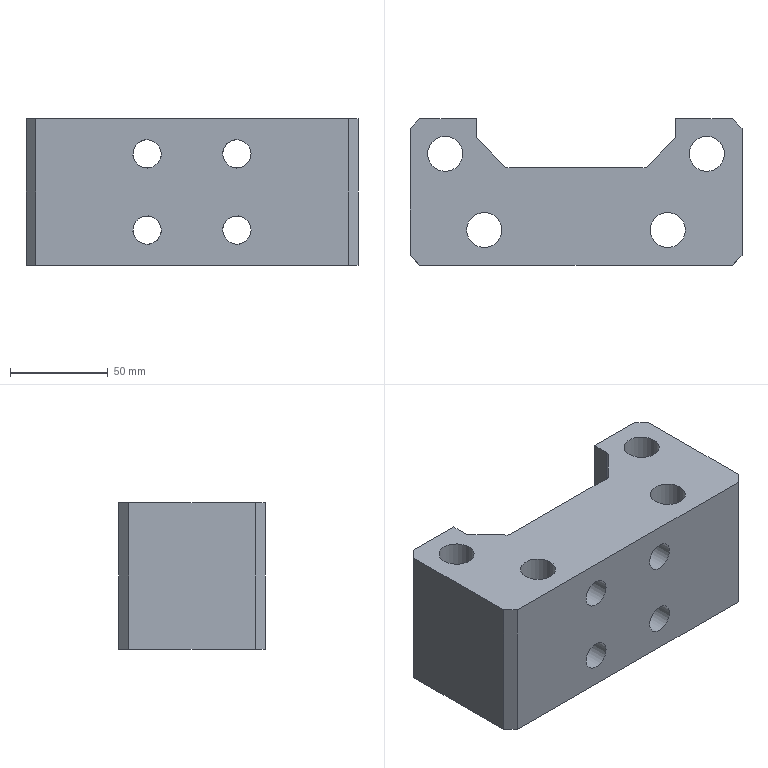Part | NX | features UB-6 2 | 1 solid | 48 faces | box 170 x 75 x 75 mm | volume 622690 mm3 | plane 22 | cylinder 20 | cone 6 | commonest cylinder face diameters 6 x4 14.5 x4 18 x4 26 x4 10.506 x2 12 x2
STEP:
#1=CARTESIAN_POINT('',(3330.594,-689.122,948.466));
#2=VERTEX_POINT('',#1);
#3=CARTESIAN_POINT('',(3330.594,-689.122,955.716));
#4=DIRECTION('',(0.,-1.,0.));
#5=DIRECTION('',(0.,0.,-1.));
#6=AXIS2_PLACEMENT_3D('',#3,#4,#5);
#7=CIRCLE('',#6,7.25);
#8=EDGE_CURVE('',#2,#2,#7,.T.);
#9=ORIENTED_EDGE('',*,*,#8,.F.);
#10=EDGE_LOOP('',(#9));
#11=FACE_BOUND('',#10,.T.);
#12=CARTESIAN_POINT('',(3284.594,-689.122,948.466));
#13=VERTEX_POINT('',#12);
#14=CARTESIAN_POINT('',(3284.594,-689.122,955.716));
#15=DIRECTION('',(0.,-1.,0.));
#16=DIRECTION('',(0.,0.,-1.));
#17=AXIS2_PLACEMENT_3D('',#14,#15,#16);
#18=CIRCLE('',#17,7.25);
#19=EDGE_CURVE('',#13,#13,#18,.T.);
#20=ORIENTED_EDGE('',*,*,#19,.F.);
#21=EDGE_LOOP('',(#20));
#22=FACE_BOUND('',#21,.T.);
#23=CARTESIAN_POINT('',(3227.594,-689.122,973.716));
#24=VERTEX_POINT('',#23);
#25=CARTESIAN_POINT('',(3387.594,-689.122,973.716));
#26=VERTEX_POINT('',#25);
#27=CARTESIAN_POINT('',(3237.747,-689.122,973.716));
#28=DIRECTION('',(1.,0.,0.));
#29=VECTOR('',#28,1000.);
#30=LINE('',#27,#29);
#31=EDGE_CURVE('',#24,#26,#30,.T.);
#32=ORIENTED_EDGE('',*,*,#31,.F.);
#33=CARTESIAN_POINT('',(3227.594,-689.122,898.716));
#34=VERTEX_POINT('',#33);
#35=CARTESIAN_POINT('',(3227.594,-689.122,973.716));
#36=DIRECTION('',(0.,0.,1.));
#37=VECTOR('',#36,1000.);
#38=LINE('',#35,#37);
#39=EDGE_CURVE('',#34,#24,#38,.T.);
#40=ORIENTED_EDGE('',*,*,#39,.F.);
#41=CARTESIAN_POINT('',(3387.594,-689.122,898.716));
#42=VERTEX_POINT('',#41);
#43=CARTESIAN_POINT('',(3645.094,-689.122,898.716));
#44=DIRECTION('',(1.,0.,0.));
#45=VECTOR('',#44,1000.);
#46=LINE('',#43,#45);
#47=EDGE_CURVE('',#34,#42,#46,.T.);
#48=ORIENTED_EDGE('',*,*,#47,.T.);
#49=CARTESIAN_POINT('',(3387.594,-689.122,1023.116));
#50=DIRECTION('',(0.,0.,-1.));
#51=VECTOR('',#50,1000.);
#52=LINE('',#49,#51);
#53=EDGE_CURVE('',#26,#42,#52,.T.);
#54=ORIENTED_EDGE('',*,*,#53,.F.);
#55=EDGE_LOOP('',(#32,#40,#48,#54));
#56=FACE_BOUND('',#55,.T.);
#57=CARTESIAN_POINT('',(3284.594,-689.122,909.466));
#58=VERTEX_POINT('',#57);
#59=CARTESIAN_POINT('',(3284.594,-689.122,916.716));
#60=DIRECTION('',(0.,-1.,0.));
#61=DIRECTION('',(0.,0.,-1.));
#62=AXIS2_PLACEMENT_3D('',#59,#60,#61);
#63=CIRCLE('',#62,7.25);
#64=EDGE_CURVE('',#58,#58,#63,.T.);
#65=ORIENTED_EDGE('',*,*,#64,.F.);
#66=EDGE_LOOP('',(#65));
#67=FACE_BOUND('',#66,.T.);
#68=CARTESIAN_POINT('',(3330.594,-689.122,909.466));
#69=VERTEX_POINT('',#68);
#70=CARTESIAN_POINT('',(3330.594,-689.122,916.716));
#71=DIRECTION('',(0.,-1.,0.));
#72=DIRECTION('',(0.,0.,-1.));
#73=AXIS2_PLACEMENT_3D('',#70,#71,#72);
#74=CIRCLE('',#73,7.25);
#75=EDGE_CURVE('',#69,#69,#74,.T.);
#76=ORIENTED_EDGE('',*,*,#75,.F.);
#77=EDGE_LOOP('',(#76));
#78=FACE_BOUND('',#77,.T.);
#79=CARTESIAN_POINT('',(4847.709,-689.122,1023.116));
#80=DIRECTION('',(0.,1.,0.));
#81=DIRECTION('',(0.,0.,-1.));
#82=AXIS2_PLACEMENT_3D('',#79,#80,#81);
#83=PLANE('',#82);
#84=ADVANCED_FACE('',(#11,#22,#56,#67,#78),#83,.F.);
#85=CARTESIAN_POINT('',(3269.594,-671.122,973.716));
#86=VERTEX_POINT('',#85);
#87=CARTESIAN_POINT('',(3260.594,-671.122,973.716));
#88=DIRECTION('',(0.,0.,-1.));
#89=DIRECTION('',(1.,0.,0.));
#90=AXIS2_PLACEMENT_3D('',#87,#88,#89);
#91=CIRCLE('',#90,9.);
#92=EDGE_CURVE('',#86,#86,#91,.T.);
#93=ORIENTED_EDGE('',*,*,#92,.T.);
#94=EDGE_LOOP('',(#93));
#95=FACE_BOUND('',#94,.T.);
#96=CARTESIAN_POINT('',(3383.594,-632.122,973.716));
#97=VERTEX_POINT('',#96);
#98=CARTESIAN_POINT('',(3374.594,-632.122,973.716));
#99=DIRECTION('',(0.,0.,-1.));
#100=DIRECTION('',(1.,0.,0.));
#101=AXIS2_PLACEMENT_3D('',#98,#99,#100);
#102=CIRCLE('',#101,9.);
#103=EDGE_CURVE('',#97,#97,#102,.T.);
#104=ORIENTED_EDGE('',*,*,#103,.T.);
#105=EDGE_LOOP('',(#104));
#106=FACE_BOUND('',#105,.T.);
#107=CARTESIAN_POINT('',(3249.594,-632.122,973.716));
#108=VERTEX_POINT('',#107);
#109=CARTESIAN_POINT('',(3240.594,-632.122,973.716));
#110=DIRECTION('',(0.,0.,-1.));
#111=DIRECTION('',(1.,0.,0.));
#112=AXIS2_PLACEMENT_3D('',#109,#110,#111);
#113=CIRCLE('',#112,9.);
#114=EDGE_CURVE('',#108,#108,#113,.T.);
#115=ORIENTED_EDGE('',*,*,#114,.T.);
#116=EDGE_LOOP('',(#115));
#117=FACE_BOUND('',#116,.T.);
#118=CARTESIAN_POINT('',(3363.594,-671.122,973.716));
#119=VERTEX_POINT('',#118);
#120=CARTESIAN_POINT('',(3354.594,-671.122,973.716));
#121=DIRECTION('',(0.,0.,-1.));
#122=DIRECTION('',(1.,0.,0.));
#123=AXIS2_PLACEMENT_3D('',#120,#121,#122);
#124=CIRCLE('',#123,9.);
#125=EDGE_CURVE('',#119,#119,#124,.T.);
#126=ORIENTED_EDGE('',*,*,#125,.T.);
#127=EDGE_LOOP('',(#126));
#128=FACE_BOUND('',#127,.T.);
#129=CARTESIAN_POINT('',(3345.075,-637.498,973.716));
#130=VERTEX_POINT('',#129);
#131=CARTESIAN_POINT('',(3341.156,-639.122,973.716));
#132=VERTEX_POINT('',#131);
#133=CARTESIAN_POINT('',(3342.304,-636.35,973.716));
#134=DIRECTION('',(0.,0.,-1.));
#135=DIRECTION('',(1.,0.,0.));
#136=AXIS2_PLACEMENT_3D('',#133,#134,#135);
#137=CIRCLE('',#136,3.);
#138=EDGE_CURVE('',#130,#132,#137,.T.);
#139=ORIENTED_EDGE('',*,*,#138,.T.);
#140=CARTESIAN_POINT('',(3274.032,-639.122,973.716));
#141=VERTEX_POINT('',#140);
#142=CARTESIAN_POINT('',(3307.594,-639.122,973.716));
#143=DIRECTION('',(1.,0.,0.));
#144=VECTOR('',#143,1000.);
#145=LINE('',#142,#144);
#146=EDGE_CURVE('',#141,#132,#145,.T.);
#147=ORIENTED_EDGE('',*,*,#146,.F.);
#148=CARTESIAN_POINT('',(3270.112,-637.498,973.716));
#149=VERTEX_POINT('',#148);
#150=CARTESIAN_POINT('',(3272.884,-636.35,973.716));
#151=DIRECTION('',(0.,0.,1.));
#152=DIRECTION('',(1.,0.,0.));
#153=AXIS2_PLACEMENT_3D('',#150,#151,#152);
#154=CIRCLE('',#153,3.);
#155=EDGE_CURVE('',#149,#141,#154,.T.);
#156=ORIENTED_EDGE('',*,*,#155,.F.);
#157=CARTESIAN_POINT('',(3257.473,-624.859,973.716));
#158=VERTEX_POINT('',#157);
#159=CARTESIAN_POINT('',(3435.992,-803.378,973.716));
#160=DIRECTION('',(-0.7071,0.7071,0.));
#161=VECTOR('',#160,1000.);
#162=LINE('',#159,#161);
#163=EDGE_CURVE('',#149,#158,#162,.T.);
#164=ORIENTED_EDGE('',*,*,#163,.T.);
#165=CARTESIAN_POINT('',(3256.594,-622.737,973.716));
#166=VERTEX_POINT('',#165);
#167=CARTESIAN_POINT('',(3259.594,-622.737,973.716));
#168=DIRECTION('',(0.,0.,1.));
#169=DIRECTION('',(1.,0.,0.));
#170=AXIS2_PLACEMENT_3D('',#167,#168,#169);
#171=CIRCLE('',#170,3.);
#172=EDGE_CURVE('',#166,#158,#171,.T.);
#173=ORIENTED_EDGE('',*,*,#172,.F.);
#174=CARTESIAN_POINT('',(3256.594,-614.122,973.716));
#175=VERTEX_POINT('',#174);
#176=CARTESIAN_POINT('',(3256.594,-1016.622,973.716));
#177=DIRECTION('',(0.,1.,0.));
#178=VECTOR('',#177,1000.);
#179=LINE('',#176,#178);
#180=EDGE_CURVE('',#166,#175,#179,.T.);
#181=ORIENTED_EDGE('',*,*,#180,.T.);
#182=CARTESIAN_POINT('',(3227.594,-614.122,973.716));
#183=VERTEX_POINT('',#182);
#184=CARTESIAN_POINT('',(4385.094,-614.122,973.716));
#185=DIRECTION('',(-1.,0.,0.));
#186=VECTOR('',#185,1000.);
#187=LINE('',#184,#186);
#188=EDGE_CURVE('',#175,#183,#187,.T.);
#189=ORIENTED_EDGE('',*,*,#188,.T.);
#190=CARTESIAN_POINT('',(3222.594,-619.122,973.716));
#191=VERTEX_POINT('',#190);
#192=CARTESIAN_POINT('',(3023.92,-817.796,973.716));
#193=DIRECTION('',(0.7071,0.7071,0.));
#194=VECTOR('',#193,1000.);
#195=LINE('',#192,#194);
#196=EDGE_CURVE('',#191,#183,#195,.T.);
#197=ORIENTED_EDGE('',*,*,#196,.F.);
#198=CARTESIAN_POINT('',(3222.594,-684.122,973.716));
#199=VERTEX_POINT('',#198);
#200=CARTESIAN_POINT('',(3222.594,-1016.622,973.716));
#201=DIRECTION('',(0.,1.,0.));
#202=VECTOR('',#201,1000.);
#203=LINE('',#200,#202);
#204=EDGE_CURVE('',#199,#191,#203,.T.);
#205=ORIENTED_EDGE('',*,*,#204,.F.);
#206=CARTESIAN_POINT('',(3388.92,-850.449,973.716));
#207=DIRECTION('',(-0.7071,0.7071,0.));
#208=VECTOR('',#207,1000.);
#209=LINE('',#206,#208);
#210=EDGE_CURVE('',#24,#199,#209,.T.);
#211=ORIENTED_EDGE('',*,*,#210,.F.);
#212=ORIENTED_EDGE('',*,*,#31,.T.);
#213=CARTESIAN_POINT('',(3392.594,-684.122,973.716));
#214=VERTEX_POINT('',#213);
#215=CARTESIAN_POINT('',(3156.42,-920.296,973.716));
#216=DIRECTION('',(-0.7071,-0.7071,0.));
#217=VECTOR('',#216,1000.);
#218=LINE('',#215,#217);
#219=EDGE_CURVE('',#214,#26,#218,.T.);
#220=ORIENTED_EDGE('',*,*,#219,.F.);
#221=CARTESIAN_POINT('',(3392.594,-619.122,973.716));
#222=VERTEX_POINT('',#221);
#223=CARTESIAN_POINT('',(3392.594,-699.122,973.716));
#224=DIRECTION('',(0.,-1.,0.));
#225=VECTOR('',#224,1000.);
#226=LINE('',#223,#225);
#227=EDGE_CURVE('',#222,#214,#226,.T.);
#228=ORIENTED_EDGE('',*,*,#227,.F.);
#229=CARTESIAN_POINT('',(3387.594,-614.122,973.716));
#230=VERTEX_POINT('',#229);
#231=CARTESIAN_POINT('',(3521.42,-747.949,973.716));
#232=DIRECTION('',(0.7071,-0.7071,0.));
#233=VECTOR('',#232,1000.);
#234=LINE('',#231,#233);
#235=EDGE_CURVE('',#230,#222,#234,.T.);
#236=ORIENTED_EDGE('',*,*,#235,.F.);
#237=CARTESIAN_POINT('',(3358.594,-614.122,973.716));
#238=VERTEX_POINT('',#237);
#239=CARTESIAN_POINT('',(4387.594,-614.122,973.716));
#240=DIRECTION('',(-1.,0.,0.));
#241=VECTOR('',#240,1000.);
#242=LINE('',#239,#241);
#243=EDGE_CURVE('',#230,#238,#242,.T.);
#244=ORIENTED_EDGE('',*,*,#243,.T.);
#245=CARTESIAN_POINT('',(3358.594,-622.737,973.716));
#246=VERTEX_POINT('',#245);
#247=CARTESIAN_POINT('',(3358.594,-656.622,973.716));
#248=DIRECTION('',(0.,1.,0.));
#249=VECTOR('',#248,1000.);
#250=LINE('',#247,#249);
#251=EDGE_CURVE('',#246,#238,#250,.T.);
#252=ORIENTED_EDGE('',*,*,#251,.F.);
#253=CARTESIAN_POINT('',(3357.715,-624.859,973.716));
#254=VERTEX_POINT('',#253);
#255=CARTESIAN_POINT('',(3355.594,-622.737,973.716));
#256=DIRECTION('',(0.,0.,1.));
#257=DIRECTION('',(1.,0.,0.));
#258=AXIS2_PLACEMENT_3D('',#255,#256,#257);
#259=CIRCLE('',#258,3.);
#260=EDGE_CURVE('',#254,#246,#259,.T.);
#261=ORIENTED_EDGE('',*,*,#260,.F.);
#262=CARTESIAN_POINT('',(3340.523,-642.051,973.716));
#263=DIRECTION('',(-0.7071,-0.7071,0.));
#264=VECTOR('',#263,1000.);
#265=LINE('',#262,#264);
#266=EDGE_CURVE('',#254,#130,#265,.T.);
#267=ORIENTED_EDGE('',*,*,#266,.T.);
#268=EDGE_LOOP('',(#139,#147,#156,#164,#173,#181,#189,#197,#205,#211,#212,#220,#228,#236,#244,#252,#261,#267));
#269=FACE_BOUND('',#268,.T.);
#270=CARTESIAN_POINT('',(3237.747,-1016.622,973.716));
#271=DIRECTION('',(0.,0.,1.));
#272=DIRECTION('',(-1.,0.,0.));
#273=AXIS2_PLACEMENT_3D('',#270,#271,#272);
#274=PLANE('',#273);
#275=ADVANCED_FACE('',(#95,#106,#117,#128,#269),#274,.T.);
#276=CARTESIAN_POINT('',(3231.594,-656.622,898.716));
#277=VERTEX_POINT('',#276);
#278=CARTESIAN_POINT('',(3237.594,-656.622,898.716));
#279=DIRECTION('',(0.,0.,-1.));
#280=DIRECTION('',(-1.,0.,0.));
#281=AXIS2_PLACEMENT_3D('',#278,#279,#280);
#282=CIRCLE('',#281,6.);
#283=EDGE_CURVE('',#277,#277,#282,.T.);
#284=ORIENTED_EDGE('',*,*,#283,.F.);
#285=EDGE_LOOP('',(#284));
#286=FACE_BOUND('',#285,.T.);
#287=CARTESIAN_POINT('',(3383.594,-656.622,898.716));
#288=VERTEX_POINT('',#287);
#289=CARTESIAN_POINT('',(3377.594,-656.622,898.716));
#290=DIRECTION('',(0.,0.,1.));
#291=DIRECTION('',(1.,0.,0.));
#292=AXIS2_PLACEMENT_3D('',#289,#290,#291);
#293=CIRCLE('',#292,6.);
#294=EDGE_CURVE('',#288,#288,#293,.T.);
#295=ORIENTED_EDGE('',*,*,#294,.T.);
#296=EDGE_LOOP('',(#295));
#297=FACE_BOUND('',#296,.T.);
#298=CARTESIAN_POINT('',(3273.594,-671.122,898.716));
#299=VERTEX_POINT('',#298);
#300=CARTESIAN_POINT('',(3260.594,-671.122,898.716));
#301=DIRECTION('',(0.,0.,-1.));
#302=DIRECTION('',(1.,0.,0.));
#303=AXIS2_PLACEMENT_3D('',#300,#301,#302);
#304=CIRCLE('',#303,13.);
#305=EDGE_CURVE('',#299,#299,#304,.T.);
#306=ORIENTED_EDGE('',*,*,#305,.F.);
#307=EDGE_LOOP('',(#306));
#308=FACE_BOUND('',#307,.T.);
#309=CARTESIAN_POINT('',(3387.594,-632.122,898.716));
#310=VERTEX_POINT('',#309);
#311=CARTESIAN_POINT('',(3374.594,-632.122,898.716));
#312=DIRECTION('',(0.,0.,-1.));
#313=DIRECTION('',(1.,0.,0.));
#314=AXIS2_PLACEMENT_3D('',#311,#312,#313);
#315=CIRCLE('',#314,13.);
#316=EDGE_CURVE('',#310,#310,#315,.T.);
#317=ORIENTED_EDGE('',*,*,#316,.F.);
#318=EDGE_LOOP('',(#317));
#319=FACE_BOUND('',#318,.T.);
#320=CARTESIAN_POINT('',(3253.594,-632.122,898.716));
#321=VERTEX_POINT('',#320);
#322=CARTESIAN_POINT('',(3240.594,-632.122,898.716));
#323=DIRECTION('',(0.,0.,-1.));
#324=DIRECTION('',(1.,0.,0.));
#325=AXIS2_PLACEMENT_3D('',#322,#323,#324);
#326=CIRCLE('',#325,13.);
#327=EDGE_CURVE('',#321,#321,#326,.T.);
#328=ORIENTED_EDGE('',*,*,#327,.F.);
#329=EDGE_LOOP('',(#328));
#330=FACE_BOUND('',#329,.T.);
#331=CARTESIAN_POINT('',(3367.594,-671.122,898.716));
#332=VERTEX_POINT('',#331);
#333=CARTESIAN_POINT('',(3354.594,-671.122,898.716));
#334=DIRECTION('',(0.,0.,-1.));
#335=DIRECTION('',(1.,0.,0.));
#336=AXIS2_PLACEMENT_3D('',#333,#334,#335);
#337=CIRCLE('',#336,13.);
#338=EDGE_CURVE('',#332,#332,#337,.T.);
#339=ORIENTED_EDGE('',*,*,#338,.F.);
#340=EDGE_LOOP('',(#339));
#341=FACE_BOUND('',#340,.T.);
#342=CARTESIAN_POINT('',(3357.715,-624.859,898.716));
#343=VERTEX_POINT('',#342);
#344=CARTESIAN_POINT('',(3345.075,-637.498,898.716));
#345=VERTEX_POINT('',#344);
#346=CARTESIAN_POINT('',(3340.523,-642.051,898.716));
#347=DIRECTION('',(-0.7071,-0.7071,0.));
#348=VECTOR('',#347,1000.);
#349=LINE('',#346,#348);
#350=EDGE_CURVE('',#343,#345,#349,.T.);
#351=ORIENTED_EDGE('',*,*,#350,.F.);
#352=CARTESIAN_POINT('',(3358.594,-622.737,898.716));
#353=VERTEX_POINT('',#352);
#354=CARTESIAN_POINT('',(3355.594,-622.737,898.716));
#355=DIRECTION('',(0.,0.,-1.));
#356=DIRECTION('',(1.,0.,0.));
#357=AXIS2_PLACEMENT_3D('',#354,#355,#356);
#358=CIRCLE('',#357,3.);
#359=EDGE_CURVE('',#353,#343,#358,.T.);
#360=ORIENTED_EDGE('',*,*,#359,.F.);
#361=CARTESIAN_POINT('',(3358.594,-614.122,898.716));
#362=VERTEX_POINT('',#361);
#363=CARTESIAN_POINT('',(3358.594,-1419.122,898.716));
#364=DIRECTION('',(0.,-1.,0.));
#365=VECTOR('',#364,1000.);
#366=LINE('',#363,#365);
#367=EDGE_CURVE('',#362,#353,#366,.T.);
#368=ORIENTED_EDGE('',*,*,#367,.F.);
#369=CARTESIAN_POINT('',(3387.594,-614.122,898.716));
#370=VERTEX_POINT('',#369);
#371=CARTESIAN_POINT('',(3660.094,-614.122,898.716));
#372=DIRECTION('',(1.,0.,0.));
#373=VECTOR('',#372,1000.);
#374=LINE('',#371,#373);
#375=EDGE_CURVE('',#362,#370,#374,.T.);
#376=ORIENTED_EDGE('',*,*,#375,.T.);
#377=CARTESIAN_POINT('',(3392.594,-619.122,898.716));
#378=VERTEX_POINT('',#377);
#379=CARTESIAN_POINT('',(3392.594,-619.122,898.716));
#380=DIRECTION('',(-0.7071,0.7071,0.));
#381=VECTOR('',#380,1000.);
#382=LINE('',#379,#381);
#383=EDGE_CURVE('',#378,#370,#382,.T.);
#384=ORIENTED_EDGE('',*,*,#383,.F.);
#385=CARTESIAN_POINT('',(3392.594,-684.122,898.716));
#386=VERTEX_POINT('',#385);
#387=CARTESIAN_POINT('',(3392.594,-1419.122,898.716));
#388=DIRECTION('',(0.,1.,0.));
#389=VECTOR('',#388,1000.);
#390=LINE('',#387,#389);
#391=EDGE_CURVE('',#386,#378,#390,.T.);
#392=ORIENTED_EDGE('',*,*,#391,.F.);
#393=CARTESIAN_POINT('',(3387.594,-689.122,898.716));
#394=DIRECTION('',(0.7071,0.7071,0.));
#395=VECTOR('',#394,1000.);
#396=LINE('',#393,#395);
#397=EDGE_CURVE('',#42,#386,#396,.T.);
#398=ORIENTED_EDGE('',*,*,#397,.F.);
#399=ORIENTED_EDGE('',*,*,#47,.F.);
#400=CARTESIAN_POINT('',(3222.594,-684.122,898.716));
#401=VERTEX_POINT('',#400);
#402=CARTESIAN_POINT('',(3222.594,-684.122,898.716));
#403=DIRECTION('',(0.7071,-0.7071,0.));
#404=VECTOR('',#403,1000.);
#405=LINE('',#402,#404);
#406=EDGE_CURVE('',#401,#34,#405,.T.);
#407=ORIENTED_EDGE('',*,*,#406,.F.);
#408=CARTESIAN_POINT('',(3222.594,-619.122,898.716));
#409=VERTEX_POINT('',#408);
#410=CARTESIAN_POINT('',(3222.594,-1419.122,898.716));
#411=DIRECTION('',(0.,1.,0.));
#412=VECTOR('',#411,1000.);
#413=LINE('',#410,#412);
#414=EDGE_CURVE('',#401,#409,#413,.T.);
#415=ORIENTED_EDGE('',*,*,#414,.T.);
#416=CARTESIAN_POINT('',(3227.594,-614.122,898.716));
#417=VERTEX_POINT('',#416);
#418=CARTESIAN_POINT('',(3227.594,-614.122,898.716));
#419=DIRECTION('',(-0.7071,-0.7071,0.));
#420=VECTOR('',#419,1000.);
#421=LINE('',#418,#420);
#422=EDGE_CURVE('',#417,#409,#421,.T.);
#423=ORIENTED_EDGE('',*,*,#422,.F.);
#424=CARTESIAN_POINT('',(3256.594,-614.122,898.716));
#425=VERTEX_POINT('',#424);
#426=CARTESIAN_POINT('',(4385.094,-614.122,898.716));
#427=DIRECTION('',(-1.,0.,0.));
#428=VECTOR('',#427,1000.);
#429=LINE('',#426,#428);
#430=EDGE_CURVE('',#425,#417,#429,.T.);
#431=ORIENTED_EDGE('',*,*,#430,.F.);
#432=CARTESIAN_POINT('',(3256.594,-622.737,898.716));
#433=VERTEX_POINT('',#432);
#434=CARTESIAN_POINT('',(3256.594,-656.622,898.716));
#435=DIRECTION('',(0.,-1.,0.));
#436=VECTOR('',#435,1000.);
#437=LINE('',#434,#436);
#438=EDGE_CURVE('',#425,#433,#437,.T.);
#439=ORIENTED_EDGE('',*,*,#438,.T.);
#440=CARTESIAN_POINT('',(3257.473,-624.859,898.716));
#441=VERTEX_POINT('',#440);
#442=CARTESIAN_POINT('',(3259.594,-622.737,898.716));
#443=DIRECTION('',(0.,0.,-1.));
#444=DIRECTION('',(1.,0.,0.));
#445=AXIS2_PLACEMENT_3D('',#442,#443,#444);
#446=CIRCLE('',#445,3.);
#447=EDGE_CURVE('',#441,#433,#446,.T.);
#448=ORIENTED_EDGE('',*,*,#447,.F.);
#449=CARTESIAN_POINT('',(3270.112,-637.498,898.716));
#450=VERTEX_POINT('',#449);
#451=CARTESIAN_POINT('',(3840.915,-1208.301,898.716));
#452=DIRECTION('',(-0.7071,0.7071,0.));
#453=VECTOR('',#452,1000.);
#454=LINE('',#451,#453);
#455=EDGE_CURVE('',#450,#441,#454,.T.);
#456=ORIENTED_EDGE('',*,*,#455,.F.);
#457=CARTESIAN_POINT('',(3274.032,-639.122,898.716));
#458=VERTEX_POINT('',#457);
#459=CARTESIAN_POINT('',(3272.884,-636.35,898.716));
#460=DIRECTION('',(0.,0.,-1.));
#461=DIRECTION('',(1.,0.,0.));
#462=AXIS2_PLACEMENT_3D('',#459,#460,#461);
#463=CIRCLE('',#462,3.);
#464=EDGE_CURVE('',#458,#450,#463,.T.);
#465=ORIENTED_EDGE('',*,*,#464,.F.);
#466=CARTESIAN_POINT('',(3341.156,-639.122,898.716));
#467=VERTEX_POINT('',#466);
#468=CARTESIAN_POINT('',(3645.094,-639.122,898.716));
#469=DIRECTION('',(-1.,0.,0.));
#470=VECTOR('',#469,1000.);
#471=LINE('',#468,#470);
#472=EDGE_CURVE('',#467,#458,#471,.T.);
#473=ORIENTED_EDGE('',*,*,#472,.F.);
#474=CARTESIAN_POINT('',(3342.304,-636.35,898.716));
#475=DIRECTION('',(0.,0.,-1.));
#476=DIRECTION('',(1.,0.,0.));
#477=AXIS2_PLACEMENT_3D('',#474,#475,#476);
#478=CIRCLE('',#477,3.);
#479=EDGE_CURVE('',#345,#467,#478,.T.);
#480=ORIENTED_EDGE('',*,*,#479,.F.);
#481=EDGE_LOOP('',(#351,#360,#368,#376,#384,#392,#398,#399,#407,#415,#423,#431,#439,#448,#456,#465,#473,#480));
#482=FACE_BOUND('',#481,.T.);
#483=CARTESIAN_POINT('',(3645.094,-1419.122,898.716));
#484=DIRECTION('',(0.,0.,1.));
#485=DIRECTION('',(-1.,0.,0.));
#486=AXIS2_PLACEMENT_3D('',#483,#484,#485);
#487=PLANE('',#486);
#488=ADVANCED_FACE('',(#286,#297,#308,#319,#330,#341,#482),#487,.F.);
#489=ORIENTED_EDGE('',*,*,#455,.T.);
#490=CARTESIAN_POINT('',(3257.473,-624.859,898.716));
#491=DIRECTION('',(0.,0.,-1.));
#492=VECTOR('',#491,1000.);
#493=LINE('',#490,#492);
#494=EDGE_CURVE('',#158,#441,#493,.T.);
#495=ORIENTED_EDGE('',*,*,#494,.F.);
#496=ORIENTED_EDGE('',*,*,#163,.F.);
#497=CARTESIAN_POINT('',(3270.112,-637.498,973.716));
#498=DIRECTION('',(0.,0.,1.));
#499=VECTOR('',#498,1000.);
#500=LINE('',#497,#499);
#501=EDGE_CURVE('',#450,#149,#500,.T.);
#502=ORIENTED_EDGE('',*,*,#501,.F.);
#503=EDGE_LOOP('',(#489,#495,#496,#502));
#504=FACE_BOUND('',#503,.T.);
#505=CARTESIAN_POINT('',(3289.665,-657.051,583.116));
#506=DIRECTION('',(-0.7071,-0.7071,0.));
#507=DIRECTION('',(0.,0.,1.));
#508=AXIS2_PLACEMENT_3D('',#505,#506,#507);
#509=PLANE('',#508);
#510=ADVANCED_FACE('',(#504),#509,.F.);
#511=CARTESIAN_POINT('',(3345.075,-637.498,898.716));
#512=DIRECTION('',(0.,0.,1.));
#513=VECTOR('',#512,1000.);
#514=LINE('',#511,#513);
#515=EDGE_CURVE('',#345,#130,#514,.T.);
#516=ORIENTED_EDGE('',*,*,#515,.T.);
#517=ORIENTED_EDGE('',*,*,#266,.F.);
#518=CARTESIAN_POINT('',(3357.715,-624.859,943.716));
#519=DIRECTION('',(0.,0.,1.));
#520=VECTOR('',#519,1000.);
#521=LINE('',#518,#520);
#522=EDGE_CURVE('',#343,#254,#521,.T.);
#523=ORIENTED_EDGE('',*,*,#522,.F.);
#524=ORIENTED_EDGE('',*,*,#350,.T.);
#525=EDGE_LOOP('',(#516,#517,#523,#524));
#526=FACE_BOUND('',#525,.T.);
#527=CARTESIAN_POINT('',(3340.523,-642.051,943.716));
#528=DIRECTION('',(-0.7071,0.7071,0.));
#529=DIRECTION('',(-0.7071,-0.7071,0.));
#530=AXIS2_PLACEMENT_3D('',#527,#528,#529);
#531=PLANE('',#530);
#532=ADVANCED_FACE('',(#526),#531,.T.);
#533=ORIENTED_EDGE('',*,*,#375,.F.);
#534=CARTESIAN_POINT('',(3358.594,-614.122,938.716));
#535=DIRECTION('',(0.,0.,-1.));
#536=VECTOR('',#535,1000.);
#537=LINE('',#534,#536);
#538=EDGE_CURVE('',#238,#362,#537,.T.);
#539=ORIENTED_EDGE('',*,*,#538,.F.);
#540=ORIENTED_EDGE('',*,*,#243,.F.);
#541=CARTESIAN_POINT('',(3387.594,-614.122,973.716));
#542=DIRECTION('',(0.,0.,1.));
#543=VECTOR('',#542,1000.);
#544=LINE('',#541,#543);
#545=EDGE_CURVE('',#370,#230,#544,.T.);
#546=ORIENTED_EDGE('',*,*,#545,.F.);
#547=EDGE_LOOP('',(#533,#539,#540,#546));
#548=FACE_BOUND('',#547,.T.);
#549=CARTESIAN_POINT('',(4387.594,-614.122,858.716));
#550=DIRECTION('',(0.,1.,0.));
#551=DIRECTION('',(-1.,0.,0.));
#552=AXIS2_PLACEMENT_3D('',#549,#550,#551);
#553=PLANE('',#552);
#554=ADVANCED_FACE('',(#548),#553,.T.);
#555=ORIENTED_EDGE('',*,*,#227,.T.);
#556=CARTESIAN_POINT('',(3392.594,-684.122,1068.116));
#557=DIRECTION('',(0.,0.,1.));
#558=VECTOR('',#557,1000.);
#559=LINE('',#556,#558);
#560=EDGE_CURVE('',#386,#214,#559,.T.);
#561=ORIENTED_EDGE('',*,*,#560,.F.);
#562=ORIENTED_EDGE('',*,*,#391,.T.);
#563=CARTESIAN_POINT('',(3392.594,-619.122,898.716));
#564=DIRECTION('',(0.,0.,-1.));
#565=VECTOR('',#564,1000.);
#566=LINE('',#563,#565);
#567=EDGE_CURVE('',#222,#378,#566,.T.);
#568=ORIENTED_EDGE('',*,*,#567,.F.);
#569=EDGE_LOOP('',(#555,#561,#562,#568));
#570=FACE_BOUND('',#569,.T.);
#571=CARTESIAN_POINT('',(3392.594,-699.122,1068.116));
#572=DIRECTION('',(-1.,0.,0.));
#573=DIRECTION('',(0.,0.,-1.));
#574=AXIS2_PLACEMENT_3D('',#571,#572,#573);
#575=PLANE('',#574);
#576=ADVANCED_FACE('',(#570),#575,.F.);
#577=ORIENTED_EDGE('',*,*,#251,.T.);
#578=ORIENTED_EDGE('',*,*,#538,.T.);
#579=ORIENTED_EDGE('',*,*,#367,.T.);
#580=CARTESIAN_POINT('',(3358.594,-622.737,938.716));
#581=DIRECTION('',(0.,0.,-1.));
#582=VECTOR('',#581,1000.);
#583=LINE('',#580,#582);
#584=EDGE_CURVE('',#246,#353,#583,.T.);
#585=ORIENTED_EDGE('',*,*,#584,.F.);
#586=EDGE_LOOP('',(#577,#578,#579,#585));
#587=FACE_BOUND('',#586,.T.);
#588=CARTESIAN_POINT('',(3358.594,-656.622,938.716));
#589=DIRECTION('',(1.,0.,0.));
#590=DIRECTION('',(0.,0.,1.));
#591=AXIS2_PLACEMENT_3D('',#588,#589,#590);
#592=PLANE('',#591);
#593=ADVANCED_FACE('',(#587),#592,.F.);
#594=ORIENTED_EDGE('',*,*,#204,.T.);
#595=CARTESIAN_POINT('',(3222.594,-619.122,1068.116));
#596=DIRECTION('',(0.,0.,1.));
#597=VECTOR('',#596,1000.);
#598=LINE('',#595,#597);
#599=EDGE_CURVE('',#409,#191,#598,.T.);
#600=ORIENTED_EDGE('',*,*,#599,.F.);
#601=ORIENTED_EDGE('',*,*,#414,.F.);
#602=CARTESIAN_POINT('',(3222.594,-684.122,898.716));
#603=DIRECTION('',(0.,0.,-1.));
#604=VECTOR('',#603,1000.);
#605=LINE('',#602,#604);
#606=EDGE_CURVE('',#199,#401,#605,.T.);
#607=ORIENTED_EDGE('',*,*,#606,.F.);
#608=EDGE_LOOP('',(#594,#600,#601,#607));
#609=FACE_BOUND('',#608,.T.);
#610=CARTESIAN_POINT('',(3222.594,-699.122,1068.116));
#611=DIRECTION('',(-1.,0.,0.));
#612=DIRECTION('',(0.,0.,-1.));
#613=AXIS2_PLACEMENT_3D('',#610,#611,#612);
#614=PLANE('',#613);
#615=ADVANCED_FACE('',(#609),#614,.T.);
#616=ORIENTED_EDGE('',*,*,#188,.F.);
#617=CARTESIAN_POINT('',(3256.594,-614.122,858.716));
#618=DIRECTION('',(0.,0.,-1.));
#619=VECTOR('',#618,1000.);
#620=LINE('',#617,#619);
#621=EDGE_CURVE('',#175,#425,#620,.T.);
#622=ORIENTED_EDGE('',*,*,#621,.T.);
#623=ORIENTED_EDGE('',*,*,#430,.T.);
#624=CARTESIAN_POINT('',(3227.594,-614.122,858.716));
#625=DIRECTION('',(0.,0.,-1.));
#626=VECTOR('',#625,1000.);
#627=LINE('',#624,#626);
#628=EDGE_CURVE('',#183,#417,#627,.T.);
#629=ORIENTED_EDGE('',*,*,#628,.F.);
#630=EDGE_LOOP('',(#616,#622,#623,#629));
#631=FACE_BOUND('',#630,.T.);
#632=CARTESIAN_POINT('',(4385.094,-614.122,858.716));
#633=DIRECTION('',(0.,1.,0.));
#634=DIRECTION('',(-1.,0.,0.));
#635=AXIS2_PLACEMENT_3D('',#632,#633,#634);
#636=PLANE('',#635);
#637=ADVANCED_FACE('',(#631),#636,.T.);
#638=ORIENTED_EDGE('',*,*,#438,.F.);
#639=ORIENTED_EDGE('',*,*,#621,.F.);
#640=ORIENTED_EDGE('',*,*,#180,.F.);
#641=CARTESIAN_POINT('',(3256.594,-622.737,998.716));
#642=DIRECTION('',(0.,0.,1.));
#643=VECTOR('',#642,1000.);
#644=LINE('',#641,#643);
#645=EDGE_CURVE('',#433,#166,#644,.T.);
#646=ORIENTED_EDGE('',*,*,#645,.F.);
#647=EDGE_LOOP('',(#638,#639,#640,#646));
#648=FACE_BOUND('',#647,.T.);
#649=CARTESIAN_POINT('',(3256.594,-656.622,938.716));
#650=DIRECTION('',(-1.,0.,0.));
#651=DIRECTION('',(0.,0.,-1.));
#652=AXIS2_PLACEMENT_3D('',#649,#650,#651);
#653=PLANE('',#652);
#654=ADVANCED_FACE('',(#648),#653,.F.);
#655=ORIENTED_EDGE('',*,*,#172,.T.);
#656=ORIENTED_EDGE('',*,*,#494,.T.);
#657=ORIENTED_EDGE('',*,*,#447,.T.);
#658=ORIENTED_EDGE('',*,*,#645,.T.);
#659=EDGE_LOOP('',(#655,#656,#657,#658));
#660=FACE_BOUND('',#659,.T.);
#661=CARTESIAN_POINT('',(3259.594,-622.737,583.116));
#662=DIRECTION('',(0.,0.,1.));
#663=DIRECTION('',(-1.,0.,0.));
#664=AXIS2_PLACEMENT_3D('',#661,#662,#663);
#665=CYLINDRICAL_SURFACE('',#664,3.);
#666=ADVANCED_FACE('',(#660),#665,.F.);
#667=ORIENTED_EDGE('',*,*,#359,.T.);
#668=ORIENTED_EDGE('',*,*,#522,.T.);
#669=ORIENTED_EDGE('',*,*,#260,.T.);
#670=ORIENTED_EDGE('',*,*,#584,.T.);
#671=EDGE_LOOP('',(#667,#668,#669,#670));
#672=FACE_BOUND('',#671,.T.);
#673=CARTESIAN_POINT('',(3355.594,-622.737,943.716));
#674=DIRECTION('',(0.,0.,1.));
#675=DIRECTION('',(-1.,0.,0.));
#676=AXIS2_PLACEMENT_3D('',#673,#674,#675);
#677=CYLINDRICAL_SURFACE('',#676,3.);
#678=ADVANCED_FACE('',(#672),#677,.F.);
#679=CARTESIAN_POINT('',(3292.594,-639.122,955.716));
#680=VERTEX_POINT('',#679);
#681=CARTESIAN_POINT('',(3284.594,-639.122,955.716));
#682=DIRECTION('',(0.,-1.,0.));
#683=DIRECTION('',(1.,0.,0.));
#684=AXIS2_PLACEMENT_3D('',#681,#682,#683);
#685=CIRCLE('',#684,8.);
#686=EDGE_CURVE('',#680,#680,#685,.T.);
#687=ORIENTED_EDGE('',*,*,#686,.T.);
#688=EDGE_LOOP('',(#687));
#689=FACE_BOUND('',#688,.T.);
#690=CARTESIAN_POINT('',(3338.594,-639.122,916.716));
#691=VERTEX_POINT('',#690);
#692=CARTESIAN_POINT('',(3330.594,-639.122,916.716));
#693=DIRECTION('',(0.,-1.,0.));
#694=DIRECTION('',(1.,0.,0.));
#695=AXIS2_PLACEMENT_3D('',#692,#693,#694);
#696=CIRCLE('',#695,8.);
#697=EDGE_CURVE('',#691,#691,#696,.T.);
#698=ORIENTED_EDGE('',*,*,#697,.T.);
#699=EDGE_LOOP('',(#698));
#700=FACE_BOUND('',#699,.T.);
#701=CARTESIAN_POINT('',(3292.594,-639.122,916.716));
#702=VERTEX_POINT('',#701);
#703=CARTESIAN_POINT('',(3284.594,-639.122,916.716));
#704=DIRECTION('',(0.,-1.,0.));
#705=DIRECTION('',(1.,0.,0.));
#706=AXIS2_PLACEMENT_3D('',#703,#704,#705);
#707=CIRCLE('',#706,8.);
#708=EDGE_CURVE('',#702,#702,#707,.T.);
#709=ORIENTED_EDGE('',*,*,#708,.T.);
#710=EDGE_LOOP('',(#709));
#711=FACE_BOUND('',#710,.T.);
#712=CARTESIAN_POINT('',(3338.594,-639.122,955.716));
#713=VERTEX_POINT('',#712);
#714=CARTESIAN_POINT('',(3330.594,-639.122,955.716));
#715=DIRECTION('',(0.,-1.,0.));
#716=DIRECTION('',(1.,0.,0.));
#717=AXIS2_PLACEMENT_3D('',#714,#715,#716);
#718=CIRCLE('',#717,8.);
#719=EDGE_CURVE('',#713,#713,#718,.T.);
#720=ORIENTED_EDGE('',*,*,#719,.T.);
#721=EDGE_LOOP('',(#720));
#722=FACE_BOUND('',#721,.T.);
#723=ORIENTED_EDGE('',*,*,#472,.T.);
#724=CARTESIAN_POINT('',(3274.032,-639.122,973.716));
#725=DIRECTION('',(0.,0.,-1.));
#726=VECTOR('',#725,1000.);
#727=LINE('',#724,#726);
#728=EDGE_CURVE('',#141,#458,#727,.T.);
#729=ORIENTED_EDGE('',*,*,#728,.F.);
#730=ORIENTED_EDGE('',*,*,#146,.T.);
#731=CARTESIAN_POINT('',(3341.156,-639.122,898.716));
#732=DIRECTION('',(0.,0.,1.));
#733=VECTOR('',#732,1000.);
#734=LINE('',#731,#733);
#735=EDGE_CURVE('',#467,#132,#734,.T.);
#736=ORIENTED_EDGE('',*,*,#735,.F.);
#737=EDGE_LOOP('',(#723,#729,#730,#736));
#738=FACE_BOUND('',#737,.T.);
#739=CARTESIAN_POINT('',(3307.594,-639.122,933.716));
#740=DIRECTION('',(0.,1.,0.));
#741=DIRECTION('',(-1.,0.,0.));
#742=AXIS2_PLACEMENT_3D('',#739,#740,#741);
#743=PLANE('',#742);
#744=ADVANCED_FACE('',(#689,#700,#711,#722,#738),#743,.T.);
#745=ORIENTED_EDGE('',*,*,#235,.T.);
#746=ORIENTED_EDGE('',*,*,#567,.T.);
#747=ORIENTED_EDGE('',*,*,#383,.T.);
#748=ORIENTED_EDGE('',*,*,#545,.T.);
#749=EDGE_LOOP('',(#745,#746,#747,#748));
#750=FACE_BOUND('',#749,.T.);
#751=CARTESIAN_POINT('',(3392.594,-619.122,1068.116));
#752=DIRECTION('',(0.7071,0.7071,0.));
#753=DIRECTION('',(0.,0.,-1.));
#754=AXIS2_PLACEMENT_3D('',#751,#752,#753);
#755=PLANE('',#754);
#756=ADVANCED_FACE('',(#750),#755,.T.);
#757=ORIENTED_EDGE('',*,*,#219,.T.);
#758=ORIENTED_EDGE('',*,*,#53,.T.);
#759=ORIENTED_EDGE('',*,*,#397,.T.);
#760=ORIENTED_EDGE('',*,*,#560,.T.);
#761=EDGE_LOOP('',(#757,#758,#759,#760));
#762=FACE_BOUND('',#761,.T.);
#763=CARTESIAN_POINT('',(3387.594,-689.122,1023.116));
#764=DIRECTION('',(-0.7071,0.7071,0.));
#765=DIRECTION('',(0.,0.,1.));
#766=AXIS2_PLACEMENT_3D('',#763,#764,#765);
#767=PLANE('',#766);
#768=ADVANCED_FACE('',(#762),#767,.F.);
#769=ORIENTED_EDGE('',*,*,#210,.T.);
#770=ORIENTED_EDGE('',*,*,#606,.T.);
#771=ORIENTED_EDGE('',*,*,#406,.T.);
#772=ORIENTED_EDGE('',*,*,#39,.T.);
#773=EDGE_LOOP('',(#769,#770,#771,#772));
#774=FACE_BOUND('',#773,.T.);
#775=CARTESIAN_POINT('',(3222.594,-684.122,1068.116));
#776=DIRECTION('',(-0.7071,-0.7071,0.));
#777=DIRECTION('',(0.,0.,-1.));
#778=AXIS2_PLACEMENT_3D('',#775,#776,#777);
#779=PLANE('',#778);
#780=ADVANCED_FACE('',(#774),#779,.T.);
#781=ORIENTED_EDGE('',*,*,#196,.T.);
#782=ORIENTED_EDGE('',*,*,#628,.T.);
#783=ORIENTED_EDGE('',*,*,#422,.T.);
#784=ORIENTED_EDGE('',*,*,#599,.T.);
#785=EDGE_LOOP('',(#781,#782,#783,#784));
#786=FACE_BOUND('',#785,.T.);
#787=CARTESIAN_POINT('',(3227.594,-614.122,858.716));
#788=DIRECTION('',(0.7071,-0.7071,0.));
#789=DIRECTION('',(0.,0.,1.));
#790=AXIS2_PLACEMENT_3D('',#787,#788,#789);
#791=PLANE('',#790);
#792=ADVANCED_FACE('',(#786),#791,.F.);
#793=ORIENTED_EDGE('',*,*,#464,.T.);
#794=ORIENTED_EDGE('',*,*,#501,.T.);
#795=ORIENTED_EDGE('',*,*,#155,.T.);
#796=ORIENTED_EDGE('',*,*,#728,.T.);
#797=EDGE_LOOP('',(#793,#794,#795,#796));
#798=FACE_BOUND('',#797,.T.);
#799=CARTESIAN_POINT('',(3272.884,-636.35,973.716));
#800=DIRECTION('',(0.,0.,-1.));
#801=DIRECTION('',(-1.,0.,0.));
#802=AXIS2_PLACEMENT_3D('',#799,#800,#801);
#803=CYLINDRICAL_SURFACE('',#802,3.);
#804=ADVANCED_FACE('',(#798),#803,.F.);
#805=ORIENTED_EDGE('',*,*,#138,.F.);
#806=ORIENTED_EDGE('',*,*,#515,.F.);
#807=ORIENTED_EDGE('',*,*,#479,.T.);
#808=ORIENTED_EDGE('',*,*,#735,.T.);
#809=EDGE_LOOP('',(#805,#806,#807,#808));
#810=FACE_BOUND('',#809,.T.);
#811=CARTESIAN_POINT('',(3342.304,-636.35,898.716));
#812=DIRECTION('',(0.,0.,1.));
#813=DIRECTION('',(-1.,0.,0.));
#814=AXIS2_PLACEMENT_3D('',#811,#812,#813);
#815=CYLINDRICAL_SURFACE('',#814,3.);
#816=ADVANCED_FACE('',(#810),#815,.F.);
#817=CARTESIAN_POINT('',(3337.844,-639.872,955.716));
#818=VERTEX_POINT('',#817);
#819=CARTESIAN_POINT('',(3330.594,-639.872,955.716));
#820=DIRECTION('',(0.,1.,0.));
#821=DIRECTION('',(1.,0.,0.));
#822=AXIS2_PLACEMENT_3D('',#819,#820,#821);
#823=CIRCLE('',#822,7.25);
#824=EDGE_CURVE('',#818,#818,#823,.T.);
#825=ORIENTED_EDGE('',*,*,#824,.T.);
#826=EDGE_LOOP('',(#825));
#827=FACE_BOUND('',#826,.T.);
#828=ORIENTED_EDGE('',*,*,#8,.T.);
#829=EDGE_LOOP('',(#828));
#830=FACE_BOUND('',#829,.T.);
#831=CARTESIAN_POINT('',(3330.594,-691.372,955.716));
#832=DIRECTION('',(0.,1.,0.));
#833=DIRECTION('',(0.,0.,1.));
#834=AXIS2_PLACEMENT_3D('',#831,#832,#833);
#835=CYLINDRICAL_SURFACE('',#834,7.25);
#836=ADVANCED_FACE('',(#827,#830),#835,.F.);
#837=ORIENTED_EDGE('',*,*,#824,.F.);
#838=EDGE_LOOP('',(#837));
#839=FACE_BOUND('',#838,.T.);
#840=ORIENTED_EDGE('',*,*,#719,.F.);
#841=EDGE_LOOP('',(#840));
#842=FACE_BOUND('',#841,.T.);
#843=CARTESIAN_POINT('',(3330.594,-639.122,955.716));
#844=DIRECTION('',(0.,1.,0.));
#845=DIRECTION('',(-1.,0.,0.));
#846=AXIS2_PLACEMENT_3D('',#843,#844,#845);
#847=CONICAL_SURFACE('',#846,8.,0.7854);
#848=ADVANCED_FACE('',(#839,#842),#847,.F.);
#849=CARTESIAN_POINT('',(3291.844,-639.872,916.716));
#850=VERTEX_POINT('',#849);
#851=CARTESIAN_POINT('',(3284.594,-639.872,916.716));
#852=DIRECTION('',(0.,1.,0.));
#853=DIRECTION('',(1.,0.,0.));
#854=AXIS2_PLACEMENT_3D('',#851,#852,#853);
#855=CIRCLE('',#854,7.25);
#856=EDGE_CURVE('',#850,#850,#855,.T.);
#857=ORIENTED_EDGE('',*,*,#856,.T.);
#858=EDGE_LOOP('',(#857));
#859=FACE_BOUND('',#858,.T.);
#860=ORIENTED_EDGE('',*,*,#64,.T.);
#861=EDGE_LOOP('',(#860));
#862=FACE_BOUND('',#861,.T.);
#863=CARTESIAN_POINT('',(3284.594,-691.372,916.716));
#864=DIRECTION('',(0.,1.,0.));
#865=DIRECTION('',(0.,0.,1.));
#866=AXIS2_PLACEMENT_3D('',#863,#864,#865);
#867=CYLINDRICAL_SURFACE('',#866,7.25);
#868=ADVANCED_FACE('',(#859,#862),#867,.F.);
#869=ORIENTED_EDGE('',*,*,#856,.F.);
#870=EDGE_LOOP('',(#869));
#871=FACE_BOUND('',#870,.T.);
#872=ORIENTED_EDGE('',*,*,#708,.F.);
#873=EDGE_LOOP('',(#872));
#874=FACE_BOUND('',#873,.T.);
#875=CARTESIAN_POINT('',(3284.594,-639.122,916.716));
#876=DIRECTION('',(0.,1.,0.));
#877=DIRECTION('',(-1.,0.,0.));
#878=AXIS2_PLACEMENT_3D('',#875,#876,#877);
#879=CONICAL_SURFACE('',#878,8.,0.7854);
#880=ADVANCED_FACE('',(#871,#874),#879,.F.);
#881=CARTESIAN_POINT('',(3337.844,-639.872,916.716));
#882=VERTEX_POINT('',#881);
#883=CARTESIAN_POINT('',(3330.594,-639.872,916.716));
#884=DIRECTION('',(0.,1.,0.));
#885=DIRECTION('',(1.,0.,0.));
#886=AXIS2_PLACEMENT_3D('',#883,#884,#885);
#887=CIRCLE('',#886,7.25);
#888=EDGE_CURVE('',#882,#882,#887,.T.);
#889=ORIENTED_EDGE('',*,*,#888,.T.);
#890=EDGE_LOOP('',(#889));
#891=FACE_BOUND('',#890,.T.);
#892=ORIENTED_EDGE('',*,*,#75,.T.);
#893=EDGE_LOOP('',(#892));
#894=FACE_BOUND('',#893,.T.);
#895=CARTESIAN_POINT('',(3330.594,-691.372,916.716));
#896=DIRECTION('',(0.,1.,0.));
#897=DIRECTION('',(0.,0.,1.));
#898=AXIS2_PLACEMENT_3D('',#895,#896,#897);
#899=CYLINDRICAL_SURFACE('',#898,7.25);
#900=ADVANCED_FACE('',(#891,#894),#899,.F.);
#901=ORIENTED_EDGE('',*,*,#888,.F.);
#902=EDGE_LOOP('',(#901));
#903=FACE_BOUND('',#902,.T.);
#904=ORIENTED_EDGE('',*,*,#697,.F.);
#905=EDGE_LOOP('',(#904));
#906=FACE_BOUND('',#905,.T.);
#907=CARTESIAN_POINT('',(3330.594,-639.122,916.716));
#908=DIRECTION('',(0.,1.,0.));
#909=DIRECTION('',(-1.,0.,0.));
#910=AXIS2_PLACEMENT_3D('',#907,#908,#909);
#911=CONICAL_SURFACE('',#910,8.,0.7854);
#912=ADVANCED_FACE('',(#903,#906),#911,.F.);
#913=CARTESIAN_POINT('',(3291.844,-639.872,955.716));
#914=VERTEX_POINT('',#913);
#915=CARTESIAN_POINT('',(3284.594,-639.872,955.716));
#916=DIRECTION('',(0.,1.,0.));
#917=DIRECTION('',(1.,0.,0.));
#918=AXIS2_PLACEMENT_3D('',#915,#916,#917);
#919=CIRCLE('',#918,7.25);
#920=EDGE_CURVE('',#914,#914,#919,.T.);
#921=ORIENTED_EDGE('',*,*,#920,.T.);
#922=EDGE_LOOP('',(#921));
#923=FACE_BOUND('',#922,.T.);
#924=ORIENTED_EDGE('',*,*,#19,.T.);
#925=EDGE_LOOP('',(#924));
#926=FACE_BOUND('',#925,.T.);
#927=CARTESIAN_POINT('',(3284.594,-691.372,955.716));
#928=DIRECTION('',(0.,1.,0.));
#929=DIRECTION('',(0.,0.,1.));
#930=AXIS2_PLACEMENT_3D('',#927,#928,#929);
#931=CYLINDRICAL_SURFACE('',#930,7.25);
#932=ADVANCED_FACE('',(#923,#926),#931,.F.);
#933=ORIENTED_EDGE('',*,*,#920,.F.);
#934=EDGE_LOOP('',(#933));
#935=FACE_BOUND('',#934,.T.);
#936=ORIENTED_EDGE('',*,*,#686,.F.);
#937=EDGE_LOOP('',(#936));
#938=FACE_BOUND('',#937,.T.);
#939=CARTESIAN_POINT('',(3284.594,-639.122,955.716));
#940=DIRECTION('',(0.,1.,0.));
#941=DIRECTION('',(-1.,0.,0.));
#942=AXIS2_PLACEMENT_3D('',#939,#940,#941);
#943=CONICAL_SURFACE('',#942,8.,0.7854);
#944=ADVANCED_FACE('',(#935,#938),#943,.F.);
#945=CARTESIAN_POINT('',(3341.594,-671.122,933.716));
#946=VERTEX_POINT('',#945);
#947=CARTESIAN_POINT('',(3354.594,-671.122,933.716));
#948=DIRECTION('',(0.,0.,1.));
#949=DIRECTION('',(-1.,0.,0.));
#950=AXIS2_PLACEMENT_3D('',#947,#948,#949);
#951=CIRCLE('',#950,13.);
#952=EDGE_CURVE('',#946,#946,#951,.T.);
#953=ORIENTED_EDGE('',*,*,#952,.T.);
#954=EDGE_LOOP('',(#953));
#955=FACE_BOUND('',#954,.T.);
#956=ORIENTED_EDGE('',*,*,#338,.T.);
#957=EDGE_LOOP('',(#956));
#958=FACE_BOUND('',#957,.T.);
#959=CARTESIAN_POINT('',(3354.594,-671.122,933.716));
#960=DIRECTION('',(0.,0.,-1.));
#961=DIRECTION('',(1.,0.,0.));
#962=AXIS2_PLACEMENT_3D('',#959,#960,#961);
#963=CYLINDRICAL_SURFACE('',#962,13.);
#964=ADVANCED_FACE('',(#955,#958),#963,.F.);
#965=ORIENTED_EDGE('',*,*,#125,.F.);
#966=EDGE_LOOP('',(#965));
#967=FACE_BOUND('',#966,.T.);
#968=CARTESIAN_POINT('',(3345.594,-671.122,933.716));
#969=VERTEX_POINT('',#968);
#970=CARTESIAN_POINT('',(3354.594,-671.122,933.716));
#971=DIRECTION('',(0.,0.,-1.));
#972=DIRECTION('',(-1.,0.,0.));
#973=AXIS2_PLACEMENT_3D('',#970,#971,#972);
#974=CIRCLE('',#973,9.);
#975=EDGE_CURVE('',#969,#969,#974,.T.);
#976=ORIENTED_EDGE('',*,*,#975,.T.);
#977=EDGE_LOOP('',(#976));
#978=FACE_BOUND('',#977,.T.);
#979=CARTESIAN_POINT('',(3354.594,-671.122,974.716));
#980=DIRECTION('',(0.,0.,-1.));
#981=DIRECTION('',(1.,0.,0.));
#982=AXIS2_PLACEMENT_3D('',#979,#980,#981);
#983=CYLINDRICAL_SURFACE('',#982,9.);
#984=ADVANCED_FACE('',(#967,#978),#983,.F.);
#985=ORIENTED_EDGE('',*,*,#975,.F.);
#986=EDGE_LOOP('',(#985));
#987=FACE_BOUND('',#986,.T.);
#988=ORIENTED_EDGE('',*,*,#952,.F.);
#989=EDGE_LOOP('',(#988));
#990=FACE_BOUND('',#989,.T.);
#991=CARTESIAN_POINT('',(3354.594,-671.122,933.716));
#992=DIRECTION('',(0.,0.,-1.));
#993=DIRECTION('',(1.,0.,0.));
#994=AXIS2_PLACEMENT_3D('',#991,#992,#993);
#995=PLANE('',#994);
#996=ADVANCED_FACE('',(#987,#990),#995,.T.);
#997=CARTESIAN_POINT('',(3227.594,-632.122,933.716));
#998=VERTEX_POINT('',#997);
#999=CARTESIAN_POINT('',(3240.594,-632.122,933.716));
#1000=DIRECTION('',(0.,0.,1.));
#1001=DIRECTION('',(-1.,0.,0.));
#1002=AXIS2_PLACEMENT_3D('',#999,#1000,#1001);
#1003=CIRCLE('',#1002,13.);
#1004=EDGE_CURVE('',#998,#998,#1003,.T.);
#1005=ORIENTED_EDGE('',*,*,#1004,.T.);
#1006=EDGE_LOOP('',(#1005));
#1007=FACE_BOUND('',#1006,.T.);
#1008=ORIENTED_EDGE('',*,*,#327,.T.);
#1009=EDGE_LOOP('',(#1008));
#1010=FACE_BOUND('',#1009,.T.);
#1011=CARTESIAN_POINT('',(3240.594,-632.122,933.716));
#1012=DIRECTION('',(0.,0.,-1.));
#1013=DIRECTION('',(1.,0.,0.));
#1014=AXIS2_PLACEMENT_3D('',#1011,#1012,#1013);
#1015=CYLINDRICAL_SURFACE('',#1014,13.);
#1016=ADVANCED_FACE('',(#1007,#1010),#1015,.F.);
#1017=ORIENTED_EDGE('',*,*,#114,.F.);
#1018=EDGE_LOOP('',(#1017));
#1019=FACE_BOUND('',#1018,.T.);
#1020=CARTESIAN_POINT('',(3231.594,-632.122,933.716));
#1021=VERTEX_POINT('',#1020);
#1022=CARTESIAN_POINT('',(3240.594,-632.122,933.716));
#1023=DIRECTION('',(0.,0.,-1.));
#1024=DIRECTION('',(-1.,0.,0.));
#1025=AXIS2_PLACEMENT_3D('',#1022,#1023,#1024);
#1026=CIRCLE('',#1025,9.);
#1027=EDGE_CURVE('',#1021,#1021,#1026,.T.);
#1028=ORIENTED_EDGE('',*,*,#1027,.T.);
#1029=EDGE_LOOP('',(#1028));
#1030=FACE_BOUND('',#1029,.T.);
#1031=CARTESIAN_POINT('',(3240.594,-632.122,974.716));
#1032=DIRECTION('',(0.,0.,-1.));
#1033=DIRECTION('',(1.,0.,0.));
#1034=AXIS2_PLACEMENT_3D('',#1031,#1032,#1033);
#1035=CYLINDRICAL_SURFACE('',#1034,9.);
#1036=ADVANCED_FACE('',(#1019,#1030),#1035,.F.);
#1037=ORIENTED_EDGE('',*,*,#1027,.F.);
#1038=EDGE_LOOP('',(#1037));
#1039=FACE_BOUND('',#1038,.T.);
#1040=ORIENTED_EDGE('',*,*,#1004,.F.);
#1041=EDGE_LOOP('',(#1040));
#1042=FACE_BOUND('',#1041,.T.);
#1043=CARTESIAN_POINT('',(3240.594,-632.122,933.716));
#1044=DIRECTION('',(0.,0.,-1.));
#1045=DIRECTION('',(1.,0.,0.));
#1046=AXIS2_PLACEMENT_3D('',#1043,#1044,#1045);
#1047=PLANE('',#1046);
#1048=ADVANCED_FACE('',(#1039,#1042),#1047,.T.);
#1049=CARTESIAN_POINT('',(3361.594,-632.122,933.716));
#1050=VERTEX_POINT('',#1049);
#1051=CARTESIAN_POINT('',(3374.594,-632.122,933.716));
#1052=DIRECTION('',(0.,0.,1.));
#1053=DIRECTION('',(-1.,0.,0.));
#1054=AXIS2_PLACEMENT_3D('',#1051,#1052,#1053);
#1055=CIRCLE('',#1054,13.);
#1056=EDGE_CURVE('',#1050,#1050,#1055,.T.);
#1057=ORIENTED_EDGE('',*,*,#1056,.T.);
#1058=EDGE_LOOP('',(#1057));
#1059=FACE_BOUND('',#1058,.T.);
#1060=ORIENTED_EDGE('',*,*,#316,.T.);
#1061=EDGE_LOOP('',(#1060));
#1062=FACE_BOUND('',#1061,.T.);
#1063=CARTESIAN_POINT('',(3374.594,-632.122,933.716));
#1064=DIRECTION('',(0.,0.,-1.));
#1065=DIRECTION('',(1.,0.,0.));
#1066=AXIS2_PLACEMENT_3D('',#1063,#1064,#1065);
#1067=CYLINDRICAL_SURFACE('',#1066,13.);
#1068=ADVANCED_FACE('',(#1059,#1062),#1067,.F.);
#1069=ORIENTED_EDGE('',*,*,#103,.F.);
#1070=EDGE_LOOP('',(#1069));
#1071=FACE_BOUND('',#1070,.T.);
#1072=CARTESIAN_POINT('',(3365.594,-632.122,933.716));
#1073=VERTEX_POINT('',#1072);
#1074=CARTESIAN_POINT('',(3374.594,-632.122,933.716));
#1075=DIRECTION('',(0.,0.,-1.));
#1076=DIRECTION('',(-1.,0.,0.));
#1077=AXIS2_PLACEMENT_3D('',#1074,#1075,#1076);
#1078=CIRCLE('',#1077,9.);
#1079=EDGE_CURVE('',#1073,#1073,#1078,.T.);
#1080=ORIENTED_EDGE('',*,*,#1079,.T.);
#1081=EDGE_LOOP('',(#1080));
#1082=FACE_BOUND('',#1081,.T.);
#1083=CARTESIAN_POINT('',(3374.594,-632.122,974.716));
#1084=DIRECTION('',(0.,0.,-1.));
#1085=DIRECTION('',(1.,0.,0.));
#1086=AXIS2_PLACEMENT_3D('',#1083,#1084,#1085);
#1087=CYLINDRICAL_SURFACE('',#1086,9.);
#1088=ADVANCED_FACE('',(#1071,#1082),#1087,.F.);
#1089=ORIENTED_EDGE('',*,*,#1079,.F.);
#1090=EDGE_LOOP('',(#1089));
#1091=FACE_BOUND('',#1090,.T.);
#1092=ORIENTED_EDGE('',*,*,#1056,.F.);
#1093=EDGE_LOOP('',(#1092));
#1094=FACE_BOUND('',#1093,.T.);
#1095=CARTESIAN_POINT('',(3374.594,-632.122,933.716));
#1096=DIRECTION('',(0.,0.,-1.));
#1097=DIRECTION('',(1.,0.,0.));
#1098=AXIS2_PLACEMENT_3D('',#1095,#1096,#1097);
#1099=PLANE('',#1098);
#1100=ADVANCED_FACE('',(#1091,#1094),#1099,.T.);
#1101=CARTESIAN_POINT('',(3247.594,-671.122,933.716));
#1102=VERTEX_POINT('',#1101);
#1103=CARTESIAN_POINT('',(3260.594,-671.122,933.716));
#1104=DIRECTION('',(0.,0.,1.));
#1105=DIRECTION('',(-1.,0.,0.));
#1106=AXIS2_PLACEMENT_3D('',#1103,#1104,#1105);
#1107=CIRCLE('',#1106,13.);
#1108=EDGE_CURVE('',#1102,#1102,#1107,.T.);
#1109=ORIENTED_EDGE('',*,*,#1108,.T.);
#1110=EDGE_LOOP('',(#1109));
#1111=FACE_BOUND('',#1110,.T.);
#1112=ORIENTED_EDGE('',*,*,#305,.T.);
#1113=EDGE_LOOP('',(#1112));
#1114=FACE_BOUND('',#1113,.T.);
#1115=CARTESIAN_POINT('',(3260.594,-671.122,933.716));
#1116=DIRECTION('',(0.,0.,-1.));
#1117=DIRECTION('',(1.,0.,0.));
#1118=AXIS2_PLACEMENT_3D('',#1115,#1116,#1117);
#1119=CYLINDRICAL_SURFACE('',#1118,13.);
#1120=ADVANCED_FACE('',(#1111,#1114),#1119,.F.);
#1121=ORIENTED_EDGE('',*,*,#92,.F.);
#1122=EDGE_LOOP('',(#1121));
#1123=FACE_BOUND('',#1122,.T.);
#1124=CARTESIAN_POINT('',(3251.594,-671.122,933.716));
#1125=VERTEX_POINT('',#1124);
#1126=CARTESIAN_POINT('',(3260.594,-671.122,933.716));
#1127=DIRECTION('',(0.,0.,-1.));
#1128=DIRECTION('',(-1.,0.,0.));
#1129=AXIS2_PLACEMENT_3D('',#1126,#1127,#1128);
#1130=CIRCLE('',#1129,9.);
#1131=EDGE_CURVE('',#1125,#1125,#1130,.T.);
#1132=ORIENTED_EDGE('',*,*,#1131,.T.);
#1133=EDGE_LOOP('',(#1132));
#1134=FACE_BOUND('',#1133,.T.);
#1135=CARTESIAN_POINT('',(3260.594,-671.122,974.716));
#1136=DIRECTION('',(0.,0.,-1.));
#1137=DIRECTION('',(1.,0.,0.));
#1138=AXIS2_PLACEMENT_3D('',#1135,#1136,#1137);
#1139=CYLINDRICAL_SURFACE('',#1138,9.);
#1140=ADVANCED_FACE('',(#1123,#1134),#1139,.F.);
#1141=ORIENTED_EDGE('',*,*,#1131,.F.);
#1142=EDGE_LOOP('',(#1141));
#1143=FACE_BOUND('',#1142,.T.);
#1144=ORIENTED_EDGE('',*,*,#1108,.F.);
#1145=EDGE_LOOP('',(#1144));
#1146=FACE_BOUND('',#1145,.T.);
#1147=CARTESIAN_POINT('',(3260.594,-671.122,933.716));
#1148=DIRECTION('',(0.,0.,-1.));
#1149=DIRECTION('',(1.,0.,0.));
#1150=AXIS2_PLACEMENT_3D('',#1147,#1148,#1149);
#1151=PLANE('',#1150);
#1152=ADVANCED_FACE('',(#1143,#1146),#1151,.T.);
#1153=CARTESIAN_POINT('',(3382.847,-656.622,904.716));
#1154=VERTEX_POINT('',#1153);
#1155=CARTESIAN_POINT('',(3377.594,-656.622,904.716));
#1156=DIRECTION('',(0.,0.,1.));
#1157=DIRECTION('',(1.,0.,0.));
#1158=AXIS2_PLACEMENT_3D('',#1155,#1156,#1157);
#1159=CIRCLE('',#1158,5.253);
#1160=EDGE_CURVE('',#1154,#1154,#1159,.T.);
#1161=ORIENTED_EDGE('',*,*,#1160,.F.);
#1162=EDGE_LOOP('',(#1161));
#1163=FACE_BOUND('',#1162,.T.);
#1164=CARTESIAN_POINT('',(3382.847,-656.622,938.716));
#1165=VERTEX_POINT('',#1164);
#1166=CARTESIAN_POINT('',(3377.594,-656.622,938.716));
#1167=DIRECTION('',(0.,0.,1.));
#1168=DIRECTION('',(1.,0.,0.));
#1169=AXIS2_PLACEMENT_3D('',#1166,#1167,#1168);
#1170=CIRCLE('',#1169,5.253);
#1171=EDGE_CURVE('',#1165,#1165,#1170,.T.);
#1172=ORIENTED_EDGE('',*,*,#1171,.T.);
#1173=EDGE_LOOP('',(#1172));
#1174=FACE_BOUND('',#1173,.T.);
#1175=CARTESIAN_POINT('',(3377.594,-656.622,898.716));
#1176=DIRECTION('',(0.,0.,1.));
#1177=DIRECTION('',(-1.,0.,0.));
#1178=AXIS2_PLACEMENT_3D('',#1175,#1176,#1177);
#1179=CYLINDRICAL_SURFACE('',#1178,5.253);
#1180=ADVANCED_FACE('',(#1163,#1174),#1179,.F.);
#1181=CARTESIAN_POINT('',(3377.594,-656.622,943.969));
#1182=VERTEX_POINT('',#1181);
#1183=VERTEX_LOOP('',#1182);
#1184=FACE_BOUND('',#1183,.T.);
#1185=ORIENTED_EDGE('',*,*,#1171,.F.);
#1186=EDGE_LOOP('',(#1185));
#1187=FACE_BOUND('',#1186,.T.);
#1188=CARTESIAN_POINT('',(3377.594,-656.622,938.716));
#1189=DIRECTION('',(0.,0.,-1.));
#1190=DIRECTION('',(1.,0.,0.));
#1191=AXIS2_PLACEMENT_3D('',#1188,#1189,#1190);
#1192=CONICAL_SURFACE('',#1191,5.253,0.7854);
#1193=ADVANCED_FACE('',(#1184,#1187),#1192,.F.);
#1194=ORIENTED_EDGE('',*,*,#1160,.T.);
#1195=EDGE_LOOP('',(#1194));
#1196=FACE_BOUND('',#1195,.T.);
#1197=CARTESIAN_POINT('',(3383.594,-656.622,904.716));
#1198=VERTEX_POINT('',#1197);
#1199=CARTESIAN_POINT('',(3377.594,-656.622,904.716));
#1200=DIRECTION('',(0.,0.,1.));
#1201=DIRECTION('',(1.,0.,0.));
#1202=AXIS2_PLACEMENT_3D('',#1199,#1200,#1201);
#1203=CIRCLE('',#1202,6.);
#1204=EDGE_CURVE('',#1198,#1198,#1203,.T.);
#1205=ORIENTED_EDGE('',*,*,#1204,.F.);
#1206=EDGE_LOOP('',(#1205));
#1207=FACE_BOUND('',#1206,.T.);
#1208=CARTESIAN_POINT('',(3377.594,-656.622,904.716));
#1209=DIRECTION('',(0.,0.,1.));
#1210=DIRECTION('',(-1.,0.,0.));
#1211=AXIS2_PLACEMENT_3D('',#1208,#1209,#1210);
#1212=PLANE('',#1211);
#1213=ADVANCED_FACE('',(#1196,#1207),#1212,.F.);
#1214=ORIENTED_EDGE('',*,*,#1204,.T.);
#1215=EDGE_LOOP('',(#1214));
#1216=FACE_BOUND('',#1215,.T.);
#1217=ORIENTED_EDGE('',*,*,#294,.F.);
#1218=EDGE_LOOP('',(#1217));
#1219=FACE_BOUND('',#1218,.T.);
#1220=CARTESIAN_POINT('',(3377.594,-656.622,898.716));
#1221=DIRECTION('',(0.,0.,1.));
#1222=DIRECTION('',(-1.,0.,0.));
#1223=AXIS2_PLACEMENT_3D('',#1220,#1221,#1222);
#1224=CYLINDRICAL_SURFACE('',#1223,6.);
#1225=ADVANCED_FACE('',(#1216,#1219),#1224,.F.);
#1226=CARTESIAN_POINT('',(3232.341,-656.622,904.716));
#1227=VERTEX_POINT('',#1226);
#1228=CARTESIAN_POINT('',(3237.594,-656.622,904.716));
#1229=DIRECTION('',(0.,0.,-1.));
#1230=DIRECTION('',(-1.,0.,0.));
#1231=AXIS2_PLACEMENT_3D('',#1228,#1229,#1230);
#1232=CIRCLE('',#1231,5.253);
#1233=EDGE_CURVE('',#1227,#1227,#1232,.T.);
#1234=ORIENTED_EDGE('',*,*,#1233,.T.);
#1235=EDGE_LOOP('',(#1234));
#1236=FACE_BOUND('',#1235,.T.);
#1237=CARTESIAN_POINT('',(3232.341,-656.622,938.716));
#1238=VERTEX_POINT('',#1237);
#1239=CARTESIAN_POINT('',(3237.594,-656.622,938.716));
#1240=DIRECTION('',(0.,0.,-1.));
#1241=DIRECTION('',(-1.,0.,0.));
#1242=AXIS2_PLACEMENT_3D('',#1239,#1240,#1241);
#1243=CIRCLE('',#1242,5.253);
#1244=EDGE_CURVE('',#1238,#1238,#1243,.T.);
#1245=ORIENTED_EDGE('',*,*,#1244,.F.);
#1246=EDGE_LOOP('',(#1245));
#1247=FACE_BOUND('',#1246,.T.);
#1248=CARTESIAN_POINT('',(3237.594,-656.622,898.716));
#1249=DIRECTION('',(0.,0.,1.));
#1250=DIRECTION('',(1.,0.,0.));
#1251=AXIS2_PLACEMENT_3D('',#1248,#1249,#1250);
#1252=CYLINDRICAL_SURFACE('',#1251,5.253);
#1253=ADVANCED_FACE('',(#1236,#1247),#1252,.F.);
#1254=CARTESIAN_POINT('',(3237.594,-656.622,943.969));
#1255=VERTEX_POINT('',#1254);
#1256=VERTEX_LOOP('',#1255);
#1257=FACE_BOUND('',#1256,.T.);
#1258=ORIENTED_EDGE('',*,*,#1244,.T.);
#1259=EDGE_LOOP('',(#1258));
#1260=FACE_BOUND('',#1259,.T.);
#1261=CARTESIAN_POINT('',(3237.594,-656.622,938.716));
#1262=DIRECTION('',(0.,0.,-1.));
#1263=DIRECTION('',(-1.,0.,0.));
#1264=AXIS2_PLACEMENT_3D('',#1261,#1262,#1263);
#1265=CONICAL_SURFACE('',#1264,5.253,0.7854);
#1266=ADVANCED_FACE('',(#1257,#1260),#1265,.F.);
#1267=ORIENTED_EDGE('',*,*,#1233,.F.);
#1268=EDGE_LOOP('',(#1267));
#1269=FACE_BOUND('',#1268,.T.);
#1270=CARTESIAN_POINT('',(3231.594,-656.622,904.716));
#1271=VERTEX_POINT('',#1270);
#1272=CARTESIAN_POINT('',(3237.594,-656.622,904.716));
#1273=DIRECTION('',(0.,0.,-1.));
#1274=DIRECTION('',(-1.,0.,0.));
#1275=AXIS2_PLACEMENT_3D('',#1272,#1273,#1274);
#1276=CIRCLE('',#1275,6.);
#1277=EDGE_CURVE('',#1271,#1271,#1276,.T.);
#1278=ORIENTED_EDGE('',*,*,#1277,.T.);
#1279=EDGE_LOOP('',(#1278));
#1280=FACE_BOUND('',#1279,.T.);
#1281=CARTESIAN_POINT('',(3237.594,-656.622,904.716));
#1282=DIRECTION('',(0.,0.,1.));
#1283=DIRECTION('',(1.,0.,0.));
#1284=AXIS2_PLACEMENT_3D('',#1281,#1282,#1283);
#1285=PLANE('',#1284);
#1286=ADVANCED_FACE('',(#1269,#1280),#1285,.F.);
#1287=ORIENTED_EDGE('',*,*,#1277,.F.);
#1288=EDGE_LOOP('',(#1287));
#1289=FACE_BOUND('',#1288,.T.);
#1290=ORIENTED_EDGE('',*,*,#283,.T.);
#1291=EDGE_LOOP('',(#1290));
#1292=FACE_BOUND('',#1291,.T.);
#1293=CARTESIAN_POINT('',(3237.594,-656.622,898.716));
#1294=DIRECTION('',(0.,0.,1.));
#1295=DIRECTION('',(1.,0.,0.));
#1296=AXIS2_PLACEMENT_3D('',#1293,#1294,#1295);
#1297=CYLINDRICAL_SURFACE('',#1296,6.);
#1298=ADVANCED_FACE('',(#1289,#1292),#1297,.F.);
#1299=CLOSED_SHELL('',(#84,#275,#488,#510,#532,#554,#576,#593,#615,#637,#654,#666,#678,#744,#756,#768,#780,#792,#804,#816,#836,#848,#868,#880,#900,#912,#932,#944,#964,#984,#996,#1016,#1036,#1048,#1068,#1088,#1100,#1120,#1140,#1152,#1180,#1193,#1213,#1225,#1253,#1266,#1286,#1298));
#1300=MANIFOLD_SOLID_BREP('',#1299);
#1301=(LENGTH_UNIT()NAMED_UNIT(*)SI_UNIT(.MILLI.,.METRE.));
#1302=UNCERTAINTY_MEASURE_WITH_UNIT(LENGTH_MEASURE(0.00001),#1301,'','');
#1303=(NAMED_UNIT(*)PLANE_ANGLE_UNIT()SI_UNIT($,.RADIAN.));
#1304=(NAMED_UNIT(*)SI_UNIT($,.STERADIAN.)SOLID_ANGLE_UNIT());
#1305=(GEOMETRIC_REPRESENTATION_CONTEXT(3)GLOBAL_UNCERTAINTY_ASSIGNED_CONTEXT((#1302))GLOBAL_UNIT_ASSIGNED_CONTEXT((#1301,#1303,#1304))REPRESENTATION_CONTEXT('',''));
#1306=ADVANCED_BREP_SHAPE_REPRESENTATION('',(#1300),#1305);